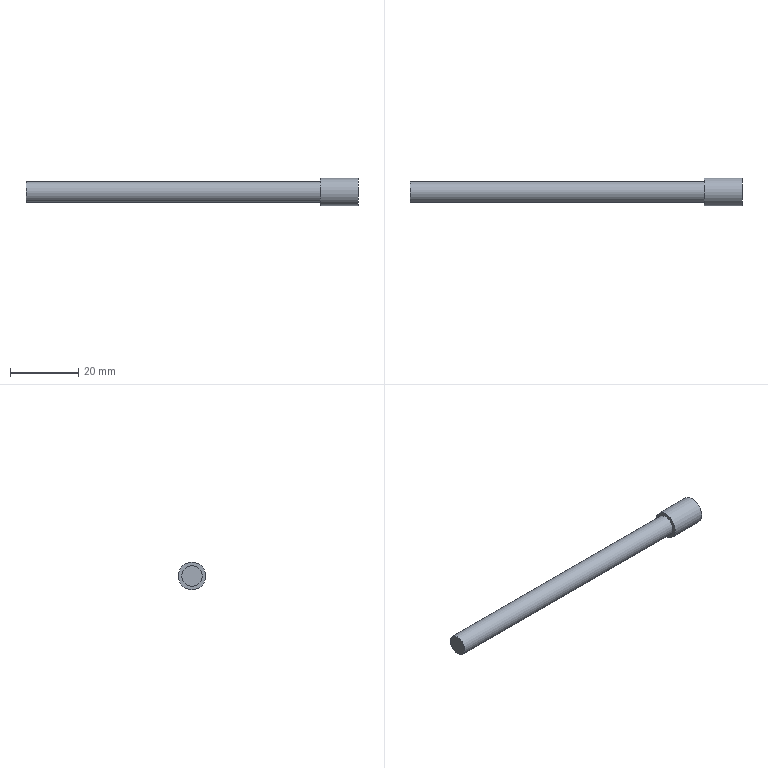Part | NX | features solid 2 | 1 solid | 5 faces | box 97 x 8 x 8 mm | volume 2985 mm3 | plane 3 | cylinder 2 | commonest cylinder face diameters 6 x1 8 x1
STEP:
#1=CARTESIAN_POINT('',(-42.,65.,-49.));
#2=VERTEX_POINT('',#1);
#3=CARTESIAN_POINT('',(-42.,65.,-52.));
#4=DIRECTION('',(1.,0.,0.));
#5=DIRECTION('',(0.,0.,1.));
#6=AXIS2_PLACEMENT_3D('',#3,#4,#5);
#7=CIRCLE('',#6,3.);
#8=EDGE_CURVE('',#2,#2,#7,.T.);
#9=ORIENTED_EDGE('',*,*,#8,.F.);
#10=EDGE_LOOP('',(#9));
#11=FACE_BOUND('',#10,.T.);
#12=CARTESIAN_POINT('',(-42.,65.,-52.));
#13=DIRECTION('',(-1.,0.,0.));
#14=DIRECTION('',(0.,0.,1.));
#15=AXIS2_PLACEMENT_3D('',#12,#13,#14);
#16=PLANE('',#15);
#17=ADVANCED_FACE('',(#11),#16,.T.);
#18=CARTESIAN_POINT('',(44.,65.,-49.));
#19=VERTEX_POINT('',#18);
#20=CARTESIAN_POINT('',(44.,65.,-52.));
#21=DIRECTION('',(-1.,0.,0.));
#22=DIRECTION('',(0.,0.,1.));
#23=AXIS2_PLACEMENT_3D('',#20,#21,#22);
#24=CIRCLE('',#23,3.);
#25=EDGE_CURVE('',#19,#19,#24,.F.);
#26=ORIENTED_EDGE('',*,*,#25,.F.);
#27=EDGE_LOOP('',(#26));
#28=FACE_BOUND('',#27,.T.);
#29=ORIENTED_EDGE('',*,*,#8,.T.);
#30=EDGE_LOOP('',(#29));
#31=FACE_BOUND('',#30,.T.);
#32=CARTESIAN_POINT('',(55.,65.,-52.));
#33=DIRECTION('',(-1.,0.,0.));
#34=DIRECTION('',(0.,0.,1.));
#35=AXIS2_PLACEMENT_3D('',#32,#33,#34);
#36=CYLINDRICAL_SURFACE('',#35,3.);
#37=ADVANCED_FACE('',(#28,#31),#36,.T.);
#38=ORIENTED_EDGE('',*,*,#25,.T.);
#39=EDGE_LOOP('',(#38));
#40=FACE_BOUND('',#39,.T.);
#41=CARTESIAN_POINT('',(44.,65.,-48.));
#42=VERTEX_POINT('',#41);
#43=CARTESIAN_POINT('',(44.,65.,-52.));
#44=DIRECTION('',(1.,0.,0.));
#45=DIRECTION('',(0.,0.,1.));
#46=AXIS2_PLACEMENT_3D('',#43,#44,#45);
#47=CIRCLE('',#46,4.);
#48=EDGE_CURVE('',#42,#42,#47,.T.);
#49=ORIENTED_EDGE('',*,*,#48,.F.);
#50=EDGE_LOOP('',(#49));
#51=FACE_BOUND('',#50,.T.);
#52=CARTESIAN_POINT('',(44.,65.,-52.));
#53=DIRECTION('',(-1.,0.,0.));
#54=DIRECTION('',(0.,0.,1.));
#55=AXIS2_PLACEMENT_3D('',#52,#53,#54);
#56=PLANE('',#55);
#57=ADVANCED_FACE('',(#40,#51),#56,.T.);
#58=ORIENTED_EDGE('',*,*,#48,.T.);
#59=EDGE_LOOP('',(#58));
#60=FACE_BOUND('',#59,.T.);
#61=CARTESIAN_POINT('',(55.,65.,-48.));
#62=VERTEX_POINT('',#61);
#63=CARTESIAN_POINT('',(55.,65.,-52.));
#64=DIRECTION('',(-1.,0.,0.));
#65=DIRECTION('',(0.,0.,1.));
#66=AXIS2_PLACEMENT_3D('',#63,#64,#65);
#67=CIRCLE('',#66,4.);
#68=EDGE_CURVE('',#62,#62,#67,.T.);
#69=ORIENTED_EDGE('',*,*,#68,.T.);
#70=EDGE_LOOP('',(#69));
#71=FACE_BOUND('',#70,.T.);
#72=CARTESIAN_POINT('',(55.,65.,-52.));
#73=DIRECTION('',(-1.,0.,0.));
#74=DIRECTION('',(0.,0.,1.));
#75=AXIS2_PLACEMENT_3D('',#72,#73,#74);
#76=CYLINDRICAL_SURFACE('',#75,4.);
#77=ADVANCED_FACE('',(#60,#71),#76,.T.);
#78=ORIENTED_EDGE('',*,*,#68,.F.);
#79=EDGE_LOOP('',(#78));
#80=FACE_BOUND('',#79,.T.);
#81=CARTESIAN_POINT('',(55.,65.,-52.));
#82=DIRECTION('',(1.,0.,0.));
#83=DIRECTION('',(0.,0.,-1.));
#84=AXIS2_PLACEMENT_3D('',#81,#82,#83);
#85=PLANE('',#84);
#86=ADVANCED_FACE('',(#80),#85,.T.);
#87=CLOSED_SHELL('',(#17,#37,#57,#77,#86));
#88=MANIFOLD_SOLID_BREP('',#87);
#89=(LENGTH_UNIT()NAMED_UNIT(*)SI_UNIT(.MILLI.,.METRE.));
#90=UNCERTAINTY_MEASURE_WITH_UNIT(LENGTH_MEASURE(0.00001),#89,'','');
#91=(NAMED_UNIT(*)PLANE_ANGLE_UNIT()SI_UNIT($,.RADIAN.));
#92=(NAMED_UNIT(*)SI_UNIT($,.STERADIAN.)SOLID_ANGLE_UNIT());
#93=(GEOMETRIC_REPRESENTATION_CONTEXT(3)GLOBAL_UNCERTAINTY_ASSIGNED_CONTEXT((#90))GLOBAL_UNIT_ASSIGNED_CONTEXT((#89,#91,#92))REPRESENTATION_CONTEXT('',''));
#94=ADVANCED_BREP_SHAPE_REPRESENTATION('',(#88),#93);